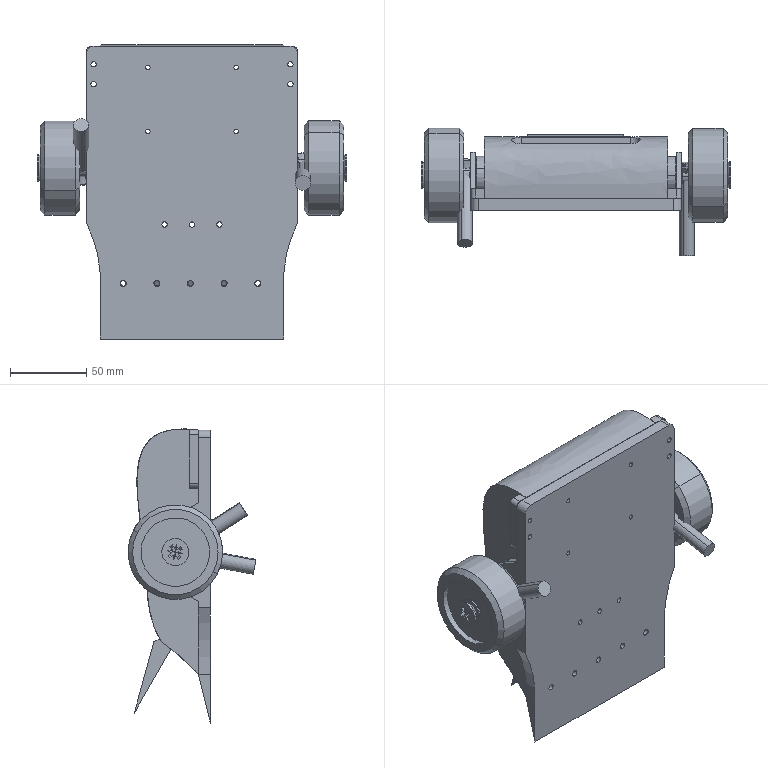Part | SolidWorks | 14 solids | 475 faces | box 202.8 x 83.824 x 192.692 mm | volume 587716 mm3 | plane 243 | cylinder 197 | cone 32 | spline 3 | commonest cylinder face diameters 3 x36 3.5 x28 12.772 x21 4 x18 0.6 x16 3.6 x10